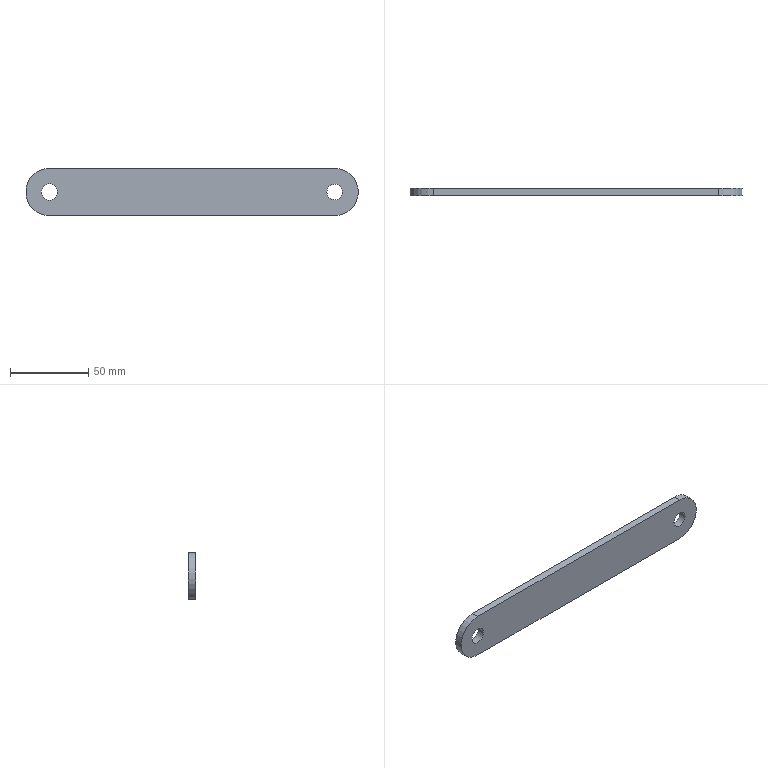Part | NX | features BREP 1 | 1 solid | 10 faces | box 212.725 x 4.763 x 30.163 mm | volume 28846 mm3 | cylinder 6 | plane 4 | commonest cylinder face diameters 10.033 x2 10.414 x2 30.163 x2
STEP:
#1=CARTESIAN_POINT('',(-91.281,0.,15.081));
#2=VERTEX_POINT('',#1);
#3=CARTESIAN_POINT('',(91.281,0.,15.081));
#4=VERTEX_POINT('',#3);
#5=CARTESIAN_POINT('',(-91.281,0.,15.081));
#6=DIRECTION('',(1.,0.,0.));
#7=VECTOR('',#6,1000.);
#8=LINE('',#5,#7);
#9=EDGE_CURVE('',#2,#4,#8,.T.);
#10=ORIENTED_EDGE('',*,*,#9,.T.);
#11=CARTESIAN_POINT('',(91.281,0.,-15.081));
#12=VERTEX_POINT('',#11);
#13=CARTESIAN_POINT('',(91.281,0.,0.));
#14=DIRECTION('',(0.,1.,0.));
#15=DIRECTION('',(0.,0.,1.));
#16=AXIS2_PLACEMENT_3D('',#13,#14,#15);
#17=CIRCLE('',#16,15.081);
#18=EDGE_CURVE('',#4,#12,#17,.T.);
#19=ORIENTED_EDGE('',*,*,#18,.T.);
#20=CARTESIAN_POINT('',(-91.281,0.,-15.081));
#21=VERTEX_POINT('',#20);
#22=CARTESIAN_POINT('',(91.281,0.,-15.081));
#23=DIRECTION('',(-1.,0.,0.));
#24=VECTOR('',#23,1000.);
#25=LINE('',#22,#24);
#26=EDGE_CURVE('',#12,#21,#25,.T.);
#27=ORIENTED_EDGE('',*,*,#26,.T.);
#28=CARTESIAN_POINT('',(-91.281,0.,0.));
#29=DIRECTION('',(0.,1.,0.));
#30=DIRECTION('',(0.,0.,-1.));
#31=AXIS2_PLACEMENT_3D('',#28,#29,#30);
#32=CIRCLE('',#31,15.081);
#33=EDGE_CURVE('',#21,#2,#32,.T.);
#34=ORIENTED_EDGE('',*,*,#33,.T.);
#35=EDGE_LOOP('',(#10,#19,#27,#34));
#36=FACE_BOUND('',#35,.T.);
#37=CARTESIAN_POINT('',(86.265,0.,0.));
#38=VERTEX_POINT('',#37);
#39=CARTESIAN_POINT('',(96.298,0.,0.));
#40=VERTEX_POINT('',#39);
#41=CARTESIAN_POINT('',(91.281,0.,0.));
#42=DIRECTION('',(0.,-1.,0.));
#43=DIRECTION('',(-1.,0.,0.));
#44=AXIS2_PLACEMENT_3D('',#41,#42,#43);
#45=CIRCLE('',#44,5.016);
#46=EDGE_CURVE('',#38,#40,#45,.T.);
#47=ORIENTED_EDGE('',*,*,#46,.T.);
#48=CARTESIAN_POINT('',(91.281,0.,0.));
#49=DIRECTION('',(0.,-1.,0.));
#50=DIRECTION('',(1.,0.,0.));
#51=AXIS2_PLACEMENT_3D('',#48,#49,#50);
#52=CIRCLE('',#51,5.016);
#53=EDGE_CURVE('',#40,#38,#52,.T.);
#54=ORIENTED_EDGE('',*,*,#53,.T.);
#55=EDGE_LOOP('',(#47,#54));
#56=FACE_BOUND('',#55,.T.);
#57=CARTESIAN_POINT('',(-96.488,0.,0.));
#58=VERTEX_POINT('',#57);
#59=CARTESIAN_POINT('',(-86.074,0.,0.));
#60=VERTEX_POINT('',#59);
#61=CARTESIAN_POINT('',(-91.281,0.,0.));
#62=DIRECTION('',(0.,-1.,0.));
#63=DIRECTION('',(-1.,0.,0.));
#64=AXIS2_PLACEMENT_3D('',#61,#62,#63);
#65=CIRCLE('',#64,5.207);
#66=EDGE_CURVE('',#58,#60,#65,.T.);
#67=ORIENTED_EDGE('',*,*,#66,.T.);
#68=CARTESIAN_POINT('',(-91.281,0.,0.));
#69=DIRECTION('',(0.,-1.,0.));
#70=DIRECTION('',(1.,0.,0.));
#71=AXIS2_PLACEMENT_3D('',#68,#69,#70);
#72=CIRCLE('',#71,5.207);
#73=EDGE_CURVE('',#60,#58,#72,.T.);
#74=ORIENTED_EDGE('',*,*,#73,.T.);
#75=EDGE_LOOP('',(#67,#74));
#76=FACE_BOUND('',#75,.T.);
#77=CARTESIAN_POINT('',(0.,0.,0.));
#78=DIRECTION('',(0.,1.,0.));
#79=DIRECTION('',(1.,0.,0.));
#80=AXIS2_PLACEMENT_3D('',#77,#78,#79);
#81=PLANE('',#80);
#82=ADVANCED_FACE('',(#36,#56,#76),#81,.T.);
#83=CARTESIAN_POINT('',(-91.281,-4.763,-15.081));
#84=VERTEX_POINT('',#83);
#85=CARTESIAN_POINT('',(-91.281,0.,-15.081));
#86=DIRECTION('',(0.,-1.,0.));
#87=VECTOR('',#86,1000.);
#88=LINE('',#85,#87);
#89=EDGE_CURVE('',#21,#84,#88,.T.);
#90=ORIENTED_EDGE('',*,*,#89,.T.);
#91=CARTESIAN_POINT('',(-91.281,-4.763,15.081));
#92=VERTEX_POINT('',#91);
#93=CARTESIAN_POINT('',(-91.281,-4.763,0.));
#94=DIRECTION('',(0.,1.,0.));
#95=DIRECTION('',(0.,0.,-1.));
#96=AXIS2_PLACEMENT_3D('',#93,#94,#95);
#97=CIRCLE('',#96,15.081);
#98=EDGE_CURVE('',#84,#92,#97,.T.);
#99=ORIENTED_EDGE('',*,*,#98,.T.);
#100=CARTESIAN_POINT('',(-91.281,0.,15.081));
#101=DIRECTION('',(0.,-1.,0.));
#102=VECTOR('',#101,1000.);
#103=LINE('',#100,#102);
#104=EDGE_CURVE('',#2,#92,#103,.T.);
#105=ORIENTED_EDGE('',*,*,#104,.F.);
#106=ORIENTED_EDGE('',*,*,#33,.F.);
#107=EDGE_LOOP('',(#90,#99,#105,#106));
#108=FACE_BOUND('',#107,.T.);
#109=CARTESIAN_POINT('',(-91.281,-2.381,0.));
#110=DIRECTION('',(0.,1.,0.));
#111=DIRECTION('',(0.,0.,-1.));
#112=AXIS2_PLACEMENT_3D('',#109,#110,#111);
#113=CYLINDRICAL_SURFACE('',#112,15.081);
#114=ADVANCED_FACE('',(#108),#113,.T.);
#115=ORIENTED_EDGE('',*,*,#104,.T.);
#116=CARTESIAN_POINT('',(91.281,-4.763,15.081));
#117=VERTEX_POINT('',#116);
#118=CARTESIAN_POINT('',(-91.281,-4.763,15.081));
#119=DIRECTION('',(1.,0.,0.));
#120=VECTOR('',#119,1000.);
#121=LINE('',#118,#120);
#122=EDGE_CURVE('',#92,#117,#121,.T.);
#123=ORIENTED_EDGE('',*,*,#122,.T.);
#124=CARTESIAN_POINT('',(91.281,0.,15.081));
#125=DIRECTION('',(0.,-1.,0.));
#126=VECTOR('',#125,1000.);
#127=LINE('',#124,#126);
#128=EDGE_CURVE('',#4,#117,#127,.T.);
#129=ORIENTED_EDGE('',*,*,#128,.F.);
#130=ORIENTED_EDGE('',*,*,#9,.F.);
#131=EDGE_LOOP('',(#115,#123,#129,#130));
#132=FACE_BOUND('',#131,.T.);
#133=CARTESIAN_POINT('',(0.,-2.381,15.081));
#134=DIRECTION('',(0.,0.,1.));
#135=DIRECTION('',(1.,0.,0.));
#136=AXIS2_PLACEMENT_3D('',#133,#134,#135);
#137=PLANE('',#136);
#138=ADVANCED_FACE('',(#132),#137,.T.);
#139=ORIENTED_EDGE('',*,*,#128,.T.);
#140=CARTESIAN_POINT('',(91.281,-4.763,-15.081));
#141=VERTEX_POINT('',#140);
#142=CARTESIAN_POINT('',(91.281,-4.763,0.));
#143=DIRECTION('',(0.,1.,0.));
#144=DIRECTION('',(0.,0.,1.));
#145=AXIS2_PLACEMENT_3D('',#142,#143,#144);
#146=CIRCLE('',#145,15.081);
#147=EDGE_CURVE('',#117,#141,#146,.T.);
#148=ORIENTED_EDGE('',*,*,#147,.T.);
#149=CARTESIAN_POINT('',(91.281,0.,-15.081));
#150=DIRECTION('',(0.,-1.,0.));
#151=VECTOR('',#150,1000.);
#152=LINE('',#149,#151);
#153=EDGE_CURVE('',#12,#141,#152,.T.);
#154=ORIENTED_EDGE('',*,*,#153,.F.);
#155=ORIENTED_EDGE('',*,*,#18,.F.);
#156=EDGE_LOOP('',(#139,#148,#154,#155));
#157=FACE_BOUND('',#156,.T.);
#158=CARTESIAN_POINT('',(91.281,-2.381,0.));
#159=DIRECTION('',(0.,1.,0.));
#160=DIRECTION('',(0.,0.,1.));
#161=AXIS2_PLACEMENT_3D('',#158,#159,#160);
#162=CYLINDRICAL_SURFACE('',#161,15.081);
#163=ADVANCED_FACE('',(#157),#162,.T.);
#164=ORIENTED_EDGE('',*,*,#153,.T.);
#165=CARTESIAN_POINT('',(91.281,-4.763,-15.081));
#166=DIRECTION('',(-1.,0.,0.));
#167=VECTOR('',#166,1000.);
#168=LINE('',#165,#167);
#169=EDGE_CURVE('',#141,#84,#168,.T.);
#170=ORIENTED_EDGE('',*,*,#169,.T.);
#171=ORIENTED_EDGE('',*,*,#89,.F.);
#172=ORIENTED_EDGE('',*,*,#26,.F.);
#173=EDGE_LOOP('',(#164,#170,#171,#172));
#174=FACE_BOUND('',#173,.T.);
#175=CARTESIAN_POINT('',(0.,-2.381,-15.081));
#176=DIRECTION('',(0.,0.,-1.));
#177=DIRECTION('',(0.,-1.,0.));
#178=AXIS2_PLACEMENT_3D('',#175,#176,#177);
#179=PLANE('',#178);
#180=ADVANCED_FACE('',(#174),#179,.T.);
#181=ORIENTED_EDGE('',*,*,#169,.F.);
#182=ORIENTED_EDGE('',*,*,#147,.F.);
#183=ORIENTED_EDGE('',*,*,#122,.F.);
#184=ORIENTED_EDGE('',*,*,#98,.F.);
#185=EDGE_LOOP('',(#181,#182,#183,#184));
#186=FACE_BOUND('',#185,.T.);
#187=CARTESIAN_POINT('',(86.265,-4.763,0.));
#188=VERTEX_POINT('',#187);
#189=CARTESIAN_POINT('',(96.298,-4.763,0.));
#190=VERTEX_POINT('',#189);
#191=CARTESIAN_POINT('',(91.281,-4.763,0.));
#192=DIRECTION('',(0.,-1.,0.));
#193=DIRECTION('',(-1.,0.,0.));
#194=AXIS2_PLACEMENT_3D('',#191,#192,#193);
#195=CIRCLE('',#194,5.016);
#196=EDGE_CURVE('',#188,#190,#195,.T.);
#197=ORIENTED_EDGE('',*,*,#196,.F.);
#198=CARTESIAN_POINT('',(91.281,-4.763,0.));
#199=DIRECTION('',(0.,-1.,0.));
#200=DIRECTION('',(1.,0.,0.));
#201=AXIS2_PLACEMENT_3D('',#198,#199,#200);
#202=CIRCLE('',#201,5.016);
#203=EDGE_CURVE('',#190,#188,#202,.T.);
#204=ORIENTED_EDGE('',*,*,#203,.F.);
#205=EDGE_LOOP('',(#197,#204));
#206=FACE_BOUND('',#205,.T.);
#207=CARTESIAN_POINT('',(-96.488,-4.763,0.));
#208=VERTEX_POINT('',#207);
#209=CARTESIAN_POINT('',(-86.074,-4.763,0.));
#210=VERTEX_POINT('',#209);
#211=CARTESIAN_POINT('',(-91.281,-4.763,0.));
#212=DIRECTION('',(0.,-1.,0.));
#213=DIRECTION('',(-1.,0.,0.));
#214=AXIS2_PLACEMENT_3D('',#211,#212,#213);
#215=CIRCLE('',#214,5.207);
#216=EDGE_CURVE('',#208,#210,#215,.T.);
#217=ORIENTED_EDGE('',*,*,#216,.F.);
#218=CARTESIAN_POINT('',(-91.281,-4.763,0.));
#219=DIRECTION('',(0.,-1.,0.));
#220=DIRECTION('',(1.,0.,0.));
#221=AXIS2_PLACEMENT_3D('',#218,#219,#220);
#222=CIRCLE('',#221,5.207);
#223=EDGE_CURVE('',#210,#208,#222,.T.);
#224=ORIENTED_EDGE('',*,*,#223,.F.);
#225=EDGE_LOOP('',(#217,#224));
#226=FACE_BOUND('',#225,.T.);
#227=CARTESIAN_POINT('',(0.,-4.763,0.));
#228=DIRECTION('',(0.,1.,0.));
#229=DIRECTION('',(1.,0.,0.));
#230=AXIS2_PLACEMENT_3D('',#227,#228,#229);
#231=PLANE('',#230);
#232=ADVANCED_FACE('',(#186,#206,#226),#231,.F.);
#233=CARTESIAN_POINT('',(96.298,0.,0.));
#234=DIRECTION('',(0.,-1.,0.));
#235=VECTOR('',#234,1000.);
#236=LINE('',#233,#235);
#237=EDGE_CURVE('',#190,#40,#236,.F.);
#238=ORIENTED_EDGE('',*,*,#237,.F.);
#239=ORIENTED_EDGE('',*,*,#203,.T.);
#240=CARTESIAN_POINT('',(86.265,0.,0.));
#241=DIRECTION('',(0.,-1.,0.));
#242=VECTOR('',#241,1000.);
#243=LINE('',#240,#242);
#244=EDGE_CURVE('',#188,#38,#243,.F.);
#245=ORIENTED_EDGE('',*,*,#244,.T.);
#246=ORIENTED_EDGE('',*,*,#53,.F.);
#247=EDGE_LOOP('',(#238,#239,#245,#246));
#248=FACE_BOUND('',#247,.T.);
#249=CARTESIAN_POINT('',(91.281,0.,0.));
#250=DIRECTION('',(0.,-1.,0.));
#251=DIRECTION('',(1.,0.,0.));
#252=AXIS2_PLACEMENT_3D('',#249,#250,#251);
#253=CYLINDRICAL_SURFACE('',#252,5.016);
#254=ADVANCED_FACE('',(#248),#253,.F.);
#255=ORIENTED_EDGE('',*,*,#244,.F.);
#256=ORIENTED_EDGE('',*,*,#196,.T.);
#257=ORIENTED_EDGE('',*,*,#237,.T.);
#258=ORIENTED_EDGE('',*,*,#46,.F.);
#259=EDGE_LOOP('',(#255,#256,#257,#258));
#260=FACE_BOUND('',#259,.T.);
#261=CARTESIAN_POINT('',(91.281,0.,0.));
#262=DIRECTION('',(0.,-1.,0.));
#263=DIRECTION('',(1.,0.,0.));
#264=AXIS2_PLACEMENT_3D('',#261,#262,#263);
#265=CYLINDRICAL_SURFACE('',#264,5.016);
#266=ADVANCED_FACE('',(#260),#265,.F.);
#267=CARTESIAN_POINT('',(-86.074,0.,0.));
#268=DIRECTION('',(0.,-1.,0.));
#269=VECTOR('',#268,1000.);
#270=LINE('',#267,#269);
#271=EDGE_CURVE('',#210,#60,#270,.F.);
#272=ORIENTED_EDGE('',*,*,#271,.F.);
#273=ORIENTED_EDGE('',*,*,#223,.T.);
#274=CARTESIAN_POINT('',(-96.488,0.,0.));
#275=DIRECTION('',(0.,-1.,0.));
#276=VECTOR('',#275,1000.);
#277=LINE('',#274,#276);
#278=EDGE_CURVE('',#208,#58,#277,.F.);
#279=ORIENTED_EDGE('',*,*,#278,.T.);
#280=ORIENTED_EDGE('',*,*,#73,.F.);
#281=EDGE_LOOP('',(#272,#273,#279,#280));
#282=FACE_BOUND('',#281,.T.);
#283=CARTESIAN_POINT('',(-91.281,0.,0.));
#284=DIRECTION('',(0.,-1.,0.));
#285=DIRECTION('',(1.,0.,0.));
#286=AXIS2_PLACEMENT_3D('',#283,#284,#285);
#287=CYLINDRICAL_SURFACE('',#286,5.207);
#288=ADVANCED_FACE('',(#282),#287,.F.);
#289=ORIENTED_EDGE('',*,*,#278,.F.);
#290=ORIENTED_EDGE('',*,*,#216,.T.);
#291=ORIENTED_EDGE('',*,*,#271,.T.);
#292=ORIENTED_EDGE('',*,*,#66,.F.);
#293=EDGE_LOOP('',(#289,#290,#291,#292));
#294=FACE_BOUND('',#293,.T.);
#295=CARTESIAN_POINT('',(-91.281,0.,0.));
#296=DIRECTION('',(0.,-1.,0.));
#297=DIRECTION('',(1.,0.,0.));
#298=AXIS2_PLACEMENT_3D('',#295,#296,#297);
#299=CYLINDRICAL_SURFACE('',#298,5.207);
#300=ADVANCED_FACE('',(#294),#299,.F.);
#301=CLOSED_SHELL('',(#82,#114,#138,#163,#180,#232,#254,#266,#288,#300));
#302=MANIFOLD_SOLID_BREP('',#301);
#303=(LENGTH_UNIT()NAMED_UNIT(*)SI_UNIT(.MILLI.,.METRE.));
#304=UNCERTAINTY_MEASURE_WITH_UNIT(LENGTH_MEASURE(0.00001),#303,'','');
#305=(NAMED_UNIT(*)PLANE_ANGLE_UNIT()SI_UNIT($,.RADIAN.));
#306=(NAMED_UNIT(*)SI_UNIT($,.STERADIAN.)SOLID_ANGLE_UNIT());
#307=(GEOMETRIC_REPRESENTATION_CONTEXT(3)GLOBAL_UNCERTAINTY_ASSIGNED_CONTEXT((#304))GLOBAL_UNIT_ASSIGNED_CONTEXT((#303,#305,#306))REPRESENTATION_CONTEXT('',''));
#308=ADVANCED_BREP_SHAPE_REPRESENTATION('',(#302),#307);